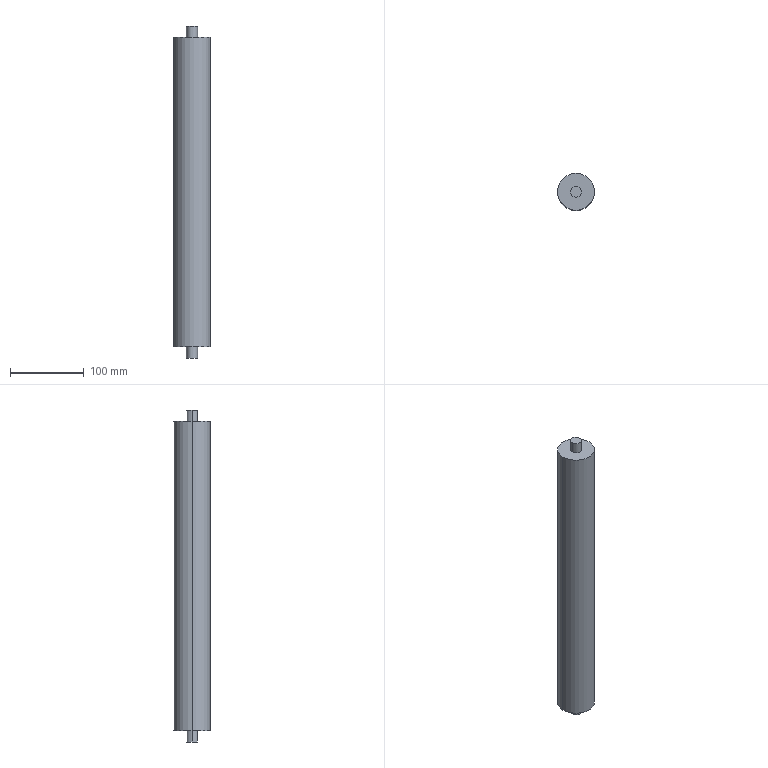Part | SolidWorks | features ICE 2, Extrusion 1 | 1 solid | 10 faces | box 50 x 50 x 450 mm | volume 829970 mm3 | cylinder 6 | plane 4 | commonest cylinder face diameters 15 x4 50 x2
STEP:
#1=CARTESIAN_POINT('',(-7.5,0.,-15.));
#2=VERTEX_POINT('',#1);
#3=CARTESIAN_POINT('',(7.5,0.,-15.));
#4=VERTEX_POINT('',#3);
#5=CARTESIAN_POINT('',(0.,0.,-15.));
#6=DIRECTION('',(0.,0.,-1.));
#7=DIRECTION('',(-1.,0.,0.));
#8=AXIS2_PLACEMENT_3D('',#5,#6,#7);
#9=CIRCLE('',#8,7.5);
#10=EDGE_CURVE('',#2,#4,#9,.T.);
#11=ORIENTED_EDGE('',*,*,#10,.F.);
#12=CARTESIAN_POINT('',(-7.5,0.,0.));
#13=VERTEX_POINT('',#12);
#14=CARTESIAN_POINT('',(-7.5,0.,-15.));
#15=DIRECTION('',(0.,0.,1.));
#16=VECTOR('',#15,1000.);
#17=LINE('',#14,#16);
#18=EDGE_CURVE('',#2,#13,#17,.T.);
#19=ORIENTED_EDGE('',*,*,#18,.T.);
#20=CARTESIAN_POINT('',(7.5,0.,0.));
#21=VERTEX_POINT('',#20);
#22=CARTESIAN_POINT('',(0.,0.,0.));
#23=DIRECTION('',(0.,0.,-1.));
#24=DIRECTION('',(-1.,0.,0.));
#25=AXIS2_PLACEMENT_3D('',#22,#23,#24);
#26=CIRCLE('',#25,7.5);
#27=EDGE_CURVE('',#13,#21,#26,.T.);
#28=ORIENTED_EDGE('',*,*,#27,.T.);
#29=CARTESIAN_POINT('',(7.5,0.,-15.));
#30=DIRECTION('',(0.,0.,1.));
#31=VECTOR('',#30,1000.);
#32=LINE('',#29,#31);
#33=EDGE_CURVE('',#4,#21,#32,.T.);
#34=ORIENTED_EDGE('',*,*,#33,.F.);
#35=EDGE_LOOP('',(#11,#19,#28,#34));
#36=FACE_OUTER_BOUND('',#35,.T.);
#37=CARTESIAN_POINT('',(0.,0.,-15.));
#38=DIRECTION('',(0.,0.,1.));
#39=DIRECTION('',(1.,0.,0.));
#40=AXIS2_PLACEMENT_3D('',#37,#38,#39);
#41=CYLINDRICAL_SURFACE('',#40,7.5);
#42=ADVANCED_FACE('',(#36),#41,.T.);
#43=CARTESIAN_POINT('',(7.5,0.,435.));
#44=VERTEX_POINT('',#43);
#45=CARTESIAN_POINT('',(-7.5,0.,435.));
#46=VERTEX_POINT('',#45);
#47=CARTESIAN_POINT('',(0.,0.,435.));
#48=DIRECTION('',(0.,0.,1.));
#49=DIRECTION('',(1.,0.,0.));
#50=AXIS2_PLACEMENT_3D('',#47,#48,#49);
#51=CIRCLE('',#50,7.5);
#52=EDGE_CURVE('',#44,#46,#51,.T.);
#53=ORIENTED_EDGE('',*,*,#52,.F.);
#54=CARTESIAN_POINT('',(7.5,0.,420.));
#55=VERTEX_POINT('',#54);
#56=CARTESIAN_POINT('',(7.5,0.,435.));
#57=DIRECTION('',(0.,0.,-1.));
#58=VECTOR('',#57,1000.);
#59=LINE('',#56,#58);
#60=EDGE_CURVE('',#44,#55,#59,.T.);
#61=ORIENTED_EDGE('',*,*,#60,.T.);
#62=CARTESIAN_POINT('',(-7.5,0.,420.));
#63=VERTEX_POINT('',#62);
#64=CARTESIAN_POINT('',(0.,0.,420.));
#65=DIRECTION('',(0.,0.,1.));
#66=DIRECTION('',(1.,0.,0.));
#67=AXIS2_PLACEMENT_3D('',#64,#65,#66);
#68=CIRCLE('',#67,7.5);
#69=EDGE_CURVE('',#55,#63,#68,.T.);
#70=ORIENTED_EDGE('',*,*,#69,.T.);
#71=CARTESIAN_POINT('',(-7.5,0.,435.));
#72=DIRECTION('',(0.,0.,-1.));
#73=VECTOR('',#72,1000.);
#74=LINE('',#71,#73);
#75=EDGE_CURVE('',#46,#63,#74,.T.);
#76=ORIENTED_EDGE('',*,*,#75,.F.);
#77=EDGE_LOOP('',(#53,#61,#70,#76));
#78=FACE_OUTER_BOUND('',#77,.T.);
#79=CARTESIAN_POINT('',(0.,0.,435.));
#80=DIRECTION('',(0.,0.,-1.));
#81=DIRECTION('',(-1.,0.,0.));
#82=AXIS2_PLACEMENT_3D('',#79,#80,#81);
#83=CYLINDRICAL_SURFACE('',#82,7.5);
#84=ADVANCED_FACE('',(#78),#83,.T.);
#85=CARTESIAN_POINT('',(25.,0.,420.));
#86=VERTEX_POINT('',#85);
#87=CARTESIAN_POINT('',(-25.,0.,420.));
#88=VERTEX_POINT('',#87);
#89=CARTESIAN_POINT('',(0.,0.,420.));
#90=DIRECTION('',(0.,0.,1.));
#91=DIRECTION('',(1.,0.,0.));
#92=AXIS2_PLACEMENT_3D('',#89,#90,#91);
#93=CIRCLE('',#92,25.);
#94=EDGE_CURVE('',#86,#88,#93,.T.);
#95=ORIENTED_EDGE('',*,*,#94,.F.);
#96=CARTESIAN_POINT('',(25.,0.,0.));
#97=VERTEX_POINT('',#96);
#98=CARTESIAN_POINT('',(25.,0.,420.));
#99=DIRECTION('',(0.,0.,-1.));
#100=VECTOR('',#99,1000.);
#101=LINE('',#98,#100);
#102=EDGE_CURVE('',#86,#97,#101,.T.);
#103=ORIENTED_EDGE('',*,*,#102,.T.);
#104=CARTESIAN_POINT('',(-25.,0.,0.));
#105=VERTEX_POINT('',#104);
#106=CARTESIAN_POINT('',(0.,0.,0.));
#107=DIRECTION('',(0.,0.,1.));
#108=DIRECTION('',(1.,0.,0.));
#109=AXIS2_PLACEMENT_3D('',#106,#107,#108);
#110=CIRCLE('',#109,25.);
#111=EDGE_CURVE('',#97,#105,#110,.T.);
#112=ORIENTED_EDGE('',*,*,#111,.T.);
#113=CARTESIAN_POINT('',(-25.,0.,420.));
#114=DIRECTION('',(0.,0.,-1.));
#115=VECTOR('',#114,1000.);
#116=LINE('',#113,#115);
#117=EDGE_CURVE('',#88,#105,#116,.T.);
#118=ORIENTED_EDGE('',*,*,#117,.F.);
#119=EDGE_LOOP('',(#95,#103,#112,#118));
#120=FACE_OUTER_BOUND('',#119,.T.);
#121=CARTESIAN_POINT('',(0.,0.,420.));
#122=DIRECTION('',(0.,0.,-1.));
#123=DIRECTION('',(-1.,0.,0.));
#124=AXIS2_PLACEMENT_3D('',#121,#122,#123);
#125=CYLINDRICAL_SURFACE('',#124,25.);
#126=ADVANCED_FACE('',(#120),#125,.T.);
#127=ORIENTED_EDGE('',*,*,#102,.F.);
#128=CARTESIAN_POINT('',(0.,0.,420.));
#129=DIRECTION('',(0.,0.,1.));
#130=DIRECTION('',(1.,0.,0.));
#131=AXIS2_PLACEMENT_3D('',#128,#129,#130);
#132=CIRCLE('',#131,25.);
#133=EDGE_CURVE('',#88,#86,#132,.T.);
#134=ORIENTED_EDGE('',*,*,#133,.F.);
#135=ORIENTED_EDGE('',*,*,#117,.T.);
#136=CARTESIAN_POINT('',(0.,0.,0.));
#137=DIRECTION('',(0.,0.,1.));
#138=DIRECTION('',(1.,0.,0.));
#139=AXIS2_PLACEMENT_3D('',#136,#137,#138);
#140=CIRCLE('',#139,25.);
#141=EDGE_CURVE('',#105,#97,#140,.T.);
#142=ORIENTED_EDGE('',*,*,#141,.T.);
#143=EDGE_LOOP('',(#127,#134,#135,#142));
#144=FACE_OUTER_BOUND('',#143,.T.);
#145=CARTESIAN_POINT('',(0.,0.,420.));
#146=DIRECTION('',(0.,0.,-1.));
#147=DIRECTION('',(-1.,0.,0.));
#148=AXIS2_PLACEMENT_3D('',#145,#146,#147);
#149=CYLINDRICAL_SURFACE('',#148,25.);
#150=ADVANCED_FACE('',(#144),#149,.T.);
#151=CARTESIAN_POINT('',(0.,0.,420.));
#152=DIRECTION('',(0.,0.,1.));
#153=DIRECTION('',(1.,0.,0.));
#154=AXIS2_PLACEMENT_3D('',#151,#152,#153);
#155=CIRCLE('',#154,7.5);
#156=EDGE_CURVE('',#63,#55,#155,.T.);
#157=ORIENTED_EDGE('',*,*,#156,.F.);
#158=ORIENTED_EDGE('',*,*,#69,.F.);
#159=EDGE_LOOP('',(#157,#158));
#160=FACE_BOUND('',#159,.T.);
#161=ORIENTED_EDGE('',*,*,#133,.T.);
#162=ORIENTED_EDGE('',*,*,#94,.T.);
#163=EDGE_LOOP('',(#161,#162));
#164=FACE_OUTER_BOUND('',#163,.T.);
#165=CARTESIAN_POINT('',(0.,0.,420.));
#166=DIRECTION('',(0.,0.,1.));
#167=DIRECTION('',(1.,0.,0.));
#168=AXIS2_PLACEMENT_3D('',#165,#166,#167);
#169=PLANE('',#168);
#170=ADVANCED_FACE('',(#160,#164),#169,.T.);
#171=CARTESIAN_POINT('',(0.,0.,0.));
#172=DIRECTION('',(0.,0.,-1.));
#173=DIRECTION('',(-1.,0.,0.));
#174=AXIS2_PLACEMENT_3D('',#171,#172,#173);
#175=CIRCLE('',#174,7.5);
#176=EDGE_CURVE('',#21,#13,#175,.T.);
#177=ORIENTED_EDGE('',*,*,#176,.F.);
#178=ORIENTED_EDGE('',*,*,#27,.F.);
#179=EDGE_LOOP('',(#177,#178));
#180=FACE_BOUND('',#179,.T.);
#181=ORIENTED_EDGE('',*,*,#141,.F.);
#182=ORIENTED_EDGE('',*,*,#111,.F.);
#183=EDGE_LOOP('',(#181,#182));
#184=FACE_OUTER_BOUND('',#183,.T.);
#185=CARTESIAN_POINT('',(0.,0.,0.));
#186=DIRECTION('',(0.,0.,1.));
#187=DIRECTION('',(1.,0.,0.));
#188=AXIS2_PLACEMENT_3D('',#185,#186,#187);
#189=PLANE('',#188);
#190=ADVANCED_FACE('',(#180,#184),#189,.F.);
#191=ORIENTED_EDGE('',*,*,#60,.F.);
#192=CARTESIAN_POINT('',(0.,0.,435.));
#193=DIRECTION('',(0.,0.,1.));
#194=DIRECTION('',(1.,0.,0.));
#195=AXIS2_PLACEMENT_3D('',#192,#193,#194);
#196=CIRCLE('',#195,7.5);
#197=EDGE_CURVE('',#46,#44,#196,.T.);
#198=ORIENTED_EDGE('',*,*,#197,.F.);
#199=ORIENTED_EDGE('',*,*,#75,.T.);
#200=ORIENTED_EDGE('',*,*,#156,.T.);
#201=EDGE_LOOP('',(#191,#198,#199,#200));
#202=FACE_OUTER_BOUND('',#201,.T.);
#203=CARTESIAN_POINT('',(0.,0.,435.));
#204=DIRECTION('',(0.,0.,-1.));
#205=DIRECTION('',(-1.,0.,0.));
#206=AXIS2_PLACEMENT_3D('',#203,#204,#205);
#207=CYLINDRICAL_SURFACE('',#206,7.5);
#208=ADVANCED_FACE('',(#202),#207,.T.);
#209=ORIENTED_EDGE('',*,*,#197,.T.);
#210=ORIENTED_EDGE('',*,*,#52,.T.);
#211=EDGE_LOOP('',(#209,#210));
#212=FACE_OUTER_BOUND('',#211,.T.);
#213=CARTESIAN_POINT('',(0.,0.,435.));
#214=DIRECTION('',(0.,0.,1.));
#215=DIRECTION('',(1.,0.,0.));
#216=AXIS2_PLACEMENT_3D('',#213,#214,#215);
#217=PLANE('',#216);
#218=ADVANCED_FACE('',(#212),#217,.T.);
#219=ORIENTED_EDGE('',*,*,#18,.F.);
#220=CARTESIAN_POINT('',(0.,0.,-15.));
#221=DIRECTION('',(0.,0.,-1.));
#222=DIRECTION('',(-1.,0.,0.));
#223=AXIS2_PLACEMENT_3D('',#220,#221,#222);
#224=CIRCLE('',#223,7.5);
#225=EDGE_CURVE('',#4,#2,#224,.T.);
#226=ORIENTED_EDGE('',*,*,#225,.F.);
#227=ORIENTED_EDGE('',*,*,#33,.T.);
#228=ORIENTED_EDGE('',*,*,#176,.T.);
#229=EDGE_LOOP('',(#219,#226,#227,#228));
#230=FACE_OUTER_BOUND('',#229,.T.);
#231=CARTESIAN_POINT('',(0.,0.,-15.));
#232=DIRECTION('',(0.,0.,1.));
#233=DIRECTION('',(1.,0.,0.));
#234=AXIS2_PLACEMENT_3D('',#231,#232,#233);
#235=CYLINDRICAL_SURFACE('',#234,7.5);
#236=ADVANCED_FACE('',(#230),#235,.T.);
#237=ORIENTED_EDGE('',*,*,#225,.T.);
#238=ORIENTED_EDGE('',*,*,#10,.T.);
#239=EDGE_LOOP('',(#237,#238));
#240=FACE_OUTER_BOUND('',#239,.T.);
#241=CARTESIAN_POINT('',(0.,0.,-15.));
#242=DIRECTION('',(0.,0.,-1.));
#243=DIRECTION('',(-1.,0.,0.));
#244=AXIS2_PLACEMENT_3D('',#241,#242,#243);
#245=PLANE('',#244);
#246=ADVANCED_FACE('',(#240),#245,.T.);
#247=CLOSED_SHELL('',(#42,#84,#126,#150,#170,#190,#208,#218,#236,#246));
#248=MANIFOLD_SOLID_BREP('',#247);
#249=CARTESIAN_POINT('',(0.,0.,0.));
#250=DIRECTION('',(0.,0.,1.));
#251=DIRECTION('',(1.,0.,0.));
#252=AXIS2_PLACEMENT_3D('',#249,#250,#251);
#253=(LENGTH_UNIT()NAMED_UNIT(*)SI_UNIT(.MILLI.,.METRE.));
#254=UNCERTAINTY_MEASURE_WITH_UNIT(LENGTH_MEASURE(0.00001),#253,'','');
#255=(NAMED_UNIT(*)PLANE_ANGLE_UNIT()SI_UNIT($,.RADIAN.));
#256=(NAMED_UNIT(*)SI_UNIT($,.STERADIAN.)SOLID_ANGLE_UNIT());
#257=(GEOMETRIC_REPRESENTATION_CONTEXT(3)GLOBAL_UNCERTAINTY_ASSIGNED_CONTEXT((#254))GLOBAL_UNIT_ASSIGNED_CONTEXT((#253,#255,#256))REPRESENTATION_CONTEXT('',''));
#258=ADVANCED_BREP_SHAPE_REPRESENTATION('',(#248,#252),#257);